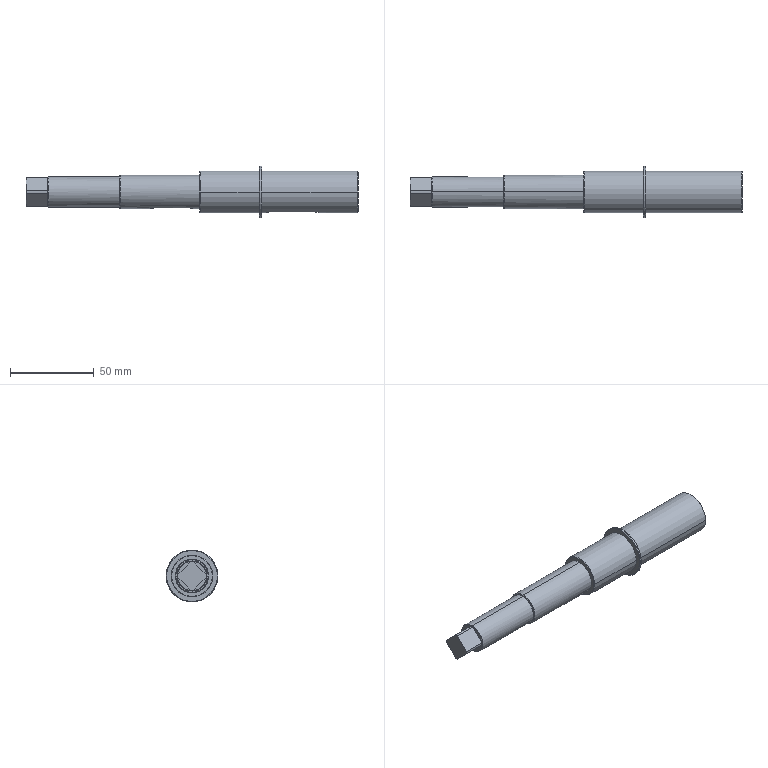Part | NX | 1 solid | 56 faces | box 198.5 x 31 x 31 mm | volume 73302 mm3 | cylinder 23 | plane 17 | cone 16 | commonest cylinder face diameters 17 x5 25 x4 6 x3 8 x3 4.2 x2 18 x2